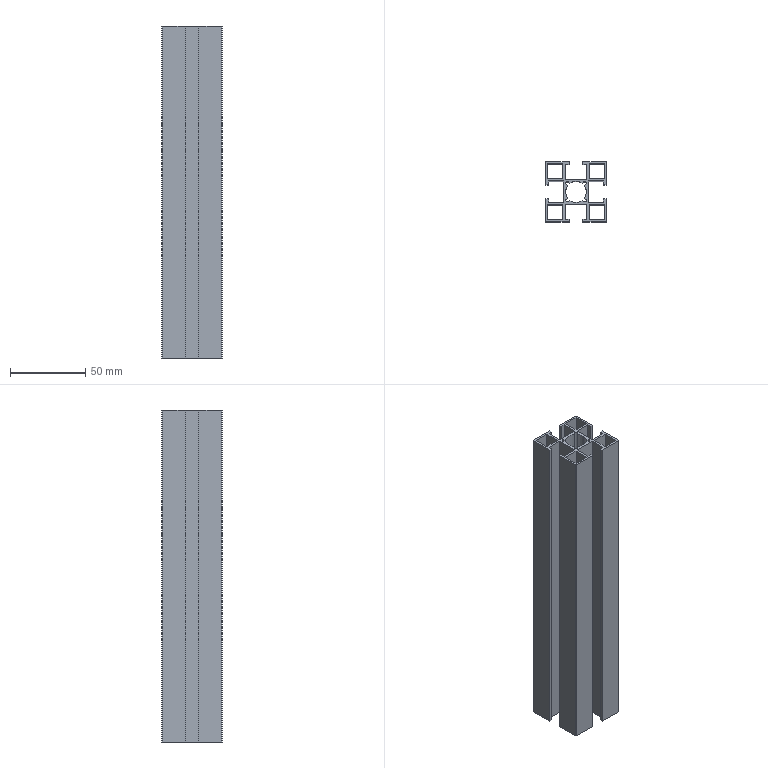Part | 1 solid | 77 faces | box 40 x 40 x 220 mm | volume 87206 mm3 | plane 62 | cylinder 15 | commonest cylinder face diameters 2.2 x6 14 x5 1 x4